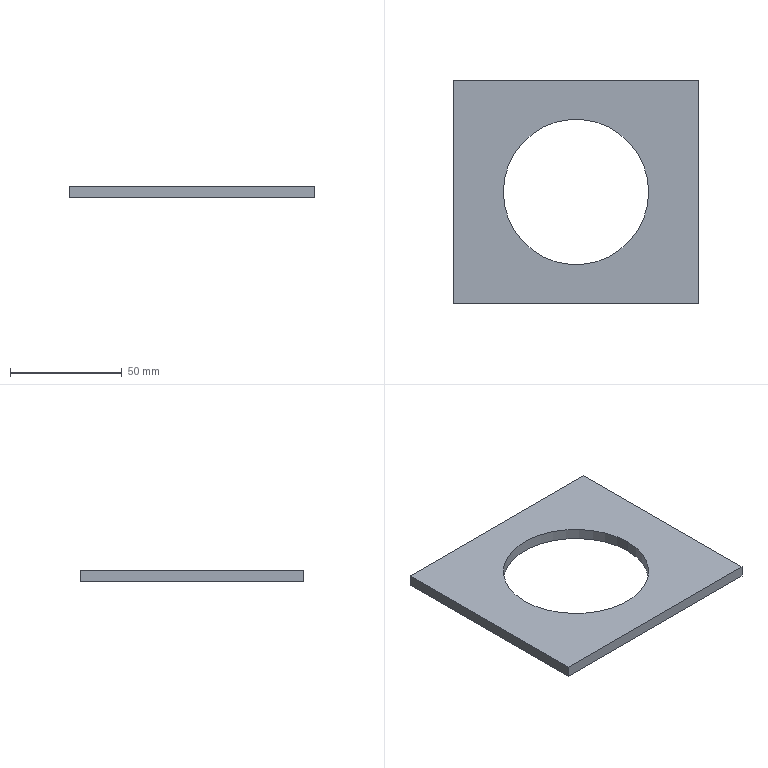Part | SolidWorks | features ICE 5, Extrusion 1 | 1 solid | 8 faces | box 110 x 100 x 5 mm | volume 38408 mm3 | plane 6 | cylinder 2 | commonest cylinder face diameters 65 x2
STEP:
#1=CARTESIAN_POINT('',(22.5,50.,0.));
#2=VERTEX_POINT('',#1);
#3=CARTESIAN_POINT('',(87.5,50.,0.));
#4=VERTEX_POINT('',#3);
#5=CARTESIAN_POINT('',(55.,50.,0.));
#6=DIRECTION('',(0.,0.,1.));
#7=DIRECTION('',(1.,0.,0.));
#8=AXIS2_PLACEMENT_3D('',#5,#6,#7);
#9=CIRCLE('',#8,32.5);
#10=EDGE_CURVE('',#2,#4,#9,.T.);
#11=ORIENTED_EDGE('',*,*,#10,.F.);
#12=CARTESIAN_POINT('',(22.5,50.,5.));
#13=VERTEX_POINT('',#12);
#14=CARTESIAN_POINT('',(22.5,50.,0.));
#15=DIRECTION('',(0.,0.,1.));
#16=VECTOR('',#15,1000.);
#17=LINE('',#14,#16);
#18=EDGE_CURVE('',#2,#13,#17,.T.);
#19=ORIENTED_EDGE('',*,*,#18,.T.);
#20=CARTESIAN_POINT('',(87.5,50.,5.));
#21=VERTEX_POINT('',#20);
#22=CARTESIAN_POINT('',(55.,50.,5.));
#23=DIRECTION('',(0.,0.,1.));
#24=DIRECTION('',(1.,0.,0.));
#25=AXIS2_PLACEMENT_3D('',#22,#23,#24);
#26=CIRCLE('',#25,32.5);
#27=EDGE_CURVE('',#13,#21,#26,.T.);
#28=ORIENTED_EDGE('',*,*,#27,.T.);
#29=CARTESIAN_POINT('',(87.5,50.,0.));
#30=DIRECTION('',(0.,0.,1.));
#31=VECTOR('',#30,1000.);
#32=LINE('',#29,#31);
#33=EDGE_CURVE('',#4,#21,#32,.T.);
#34=ORIENTED_EDGE('',*,*,#33,.F.);
#35=EDGE_LOOP('',(#11,#19,#28,#34));
#36=FACE_OUTER_BOUND('',#35,.T.);
#37=CARTESIAN_POINT('',(55.,50.,0.));
#38=DIRECTION('',(0.,0.,1.));
#39=DIRECTION('',(1.,0.,0.));
#40=AXIS2_PLACEMENT_3D('',#37,#38,#39);
#41=CYLINDRICAL_SURFACE('',#40,32.5);
#42=ADVANCED_FACE('',(#36),#41,.F.);
#43=CARTESIAN_POINT('',(0.,0.,0.));
#44=VERTEX_POINT('',#43);
#45=CARTESIAN_POINT('',(0.,0.,5.));
#46=VERTEX_POINT('',#45);
#47=CARTESIAN_POINT('',(0.,0.,0.));
#48=DIRECTION('',(0.,0.,1.));
#49=VECTOR('',#48,1000.);
#50=LINE('',#47,#49);
#51=EDGE_CURVE('',#44,#46,#50,.T.);
#52=ORIENTED_EDGE('',*,*,#51,.F.);
#53=CARTESIAN_POINT('',(110.,0.,0.));
#54=VERTEX_POINT('',#53);
#55=CARTESIAN_POINT('',(0.,0.,0.));
#56=DIRECTION('',(1.,0.,0.));
#57=VECTOR('',#56,1000.);
#58=LINE('',#55,#57);
#59=EDGE_CURVE('',#44,#54,#58,.T.);
#60=ORIENTED_EDGE('',*,*,#59,.T.);
#61=CARTESIAN_POINT('',(110.,0.,5.));
#62=VERTEX_POINT('',#61);
#63=CARTESIAN_POINT('',(110.,0.,5.));
#64=DIRECTION('',(0.,0.,-1.));
#65=VECTOR('',#64,1000.);
#66=LINE('',#63,#65);
#67=EDGE_CURVE('',#62,#54,#66,.T.);
#68=ORIENTED_EDGE('',*,*,#67,.F.);
#69=CARTESIAN_POINT('',(0.,0.,5.));
#70=DIRECTION('',(1.,0.,0.));
#71=VECTOR('',#70,1000.);
#72=LINE('',#69,#71);
#73=EDGE_CURVE('',#46,#62,#72,.T.);
#74=ORIENTED_EDGE('',*,*,#73,.F.);
#75=EDGE_LOOP('',(#52,#60,#68,#74));
#76=FACE_OUTER_BOUND('',#75,.T.);
#77=CARTESIAN_POINT('',(0.,0.,5.));
#78=DIRECTION('',(0.,1.,0.));
#79=DIRECTION('',(0.,0.,1.));
#80=AXIS2_PLACEMENT_3D('',#77,#78,#79);
#81=PLANE('',#80);
#82=ADVANCED_FACE('',(#76),#81,.F.);
#83=CARTESIAN_POINT('',(0.,100.,5.));
#84=VERTEX_POINT('',#83);
#85=CARTESIAN_POINT('',(0.,100.,0.));
#86=VERTEX_POINT('',#85);
#87=CARTESIAN_POINT('',(0.,100.,5.));
#88=DIRECTION('',(0.,0.,-1.));
#89=VECTOR('',#88,1000.);
#90=LINE('',#87,#89);
#91=EDGE_CURVE('',#84,#86,#90,.T.);
#92=ORIENTED_EDGE('',*,*,#91,.F.);
#93=CARTESIAN_POINT('',(110.,100.,5.));
#94=VERTEX_POINT('',#93);
#95=CARTESIAN_POINT('',(110.,100.,5.));
#96=DIRECTION('',(-1.,0.,0.));
#97=VECTOR('',#96,1000.);
#98=LINE('',#95,#97);
#99=EDGE_CURVE('',#94,#84,#98,.T.);
#100=ORIENTED_EDGE('',*,*,#99,.F.);
#101=CARTESIAN_POINT('',(110.,100.,0.));
#102=VERTEX_POINT('',#101);
#103=CARTESIAN_POINT('',(110.,100.,0.));
#104=DIRECTION('',(0.,0.,1.));
#105=VECTOR('',#104,1000.);
#106=LINE('',#103,#105);
#107=EDGE_CURVE('',#102,#94,#106,.T.);
#108=ORIENTED_EDGE('',*,*,#107,.F.);
#109=CARTESIAN_POINT('',(110.,100.,0.));
#110=DIRECTION('',(-1.,0.,0.));
#111=VECTOR('',#110,1000.);
#112=LINE('',#109,#111);
#113=EDGE_CURVE('',#102,#86,#112,.T.);
#114=ORIENTED_EDGE('',*,*,#113,.T.);
#115=EDGE_LOOP('',(#92,#100,#108,#114));
#116=FACE_OUTER_BOUND('',#115,.T.);
#117=CARTESIAN_POINT('',(110.,100.,5.));
#118=DIRECTION('',(0.,-1.,0.));
#119=DIRECTION('',(0.,0.,-1.));
#120=AXIS2_PLACEMENT_3D('',#117,#118,#119);
#121=PLANE('',#120);
#122=ADVANCED_FACE('',(#116),#121,.F.);
#123=CARTESIAN_POINT('',(55.,50.,5.));
#124=DIRECTION('',(0.,0.,1.));
#125=DIRECTION('',(1.,0.,0.));
#126=AXIS2_PLACEMENT_3D('',#123,#124,#125);
#127=CIRCLE('',#126,32.5);
#128=EDGE_CURVE('',#21,#13,#127,.T.);
#129=ORIENTED_EDGE('',*,*,#128,.F.);
#130=ORIENTED_EDGE('',*,*,#27,.F.);
#131=EDGE_LOOP('',(#129,#130));
#132=FACE_BOUND('',#131,.T.);
#133=ORIENTED_EDGE('',*,*,#99,.T.);
#134=CARTESIAN_POINT('',(0.,0.,5.));
#135=DIRECTION('',(0.,1.,0.));
#136=VECTOR('',#135,1000.);
#137=LINE('',#134,#136);
#138=EDGE_CURVE('',#46,#84,#137,.T.);
#139=ORIENTED_EDGE('',*,*,#138,.F.);
#140=ORIENTED_EDGE('',*,*,#73,.T.);
#141=CARTESIAN_POINT('',(110.,100.,5.));
#142=DIRECTION('',(0.,-1.,0.));
#143=VECTOR('',#142,1000.);
#144=LINE('',#141,#143);
#145=EDGE_CURVE('',#94,#62,#144,.T.);
#146=ORIENTED_EDGE('',*,*,#145,.F.);
#147=EDGE_LOOP('',(#133,#139,#140,#146));
#148=FACE_OUTER_BOUND('',#147,.T.);
#149=CARTESIAN_POINT('',(0.,0.,5.));
#150=DIRECTION('',(0.,0.,1.));
#151=DIRECTION('',(1.,0.,0.));
#152=AXIS2_PLACEMENT_3D('',#149,#150,#151);
#153=PLANE('',#152);
#154=ADVANCED_FACE('',(#132,#148),#153,.T.);
#155=CARTESIAN_POINT('',(55.,50.,0.));
#156=DIRECTION('',(0.,0.,1.));
#157=DIRECTION('',(1.,0.,0.));
#158=AXIS2_PLACEMENT_3D('',#155,#156,#157);
#159=CIRCLE('',#158,32.5);
#160=EDGE_CURVE('',#4,#2,#159,.T.);
#161=ORIENTED_EDGE('',*,*,#160,.T.);
#162=ORIENTED_EDGE('',*,*,#10,.T.);
#163=EDGE_LOOP('',(#161,#162));
#164=FACE_BOUND('',#163,.T.);
#165=CARTESIAN_POINT('',(0.,100.,0.));
#166=DIRECTION('',(0.,-1.,0.));
#167=VECTOR('',#166,1000.);
#168=LINE('',#165,#167);
#169=EDGE_CURVE('',#86,#44,#168,.T.);
#170=ORIENTED_EDGE('',*,*,#169,.F.);
#171=ORIENTED_EDGE('',*,*,#113,.F.);
#172=CARTESIAN_POINT('',(110.,0.,0.));
#173=DIRECTION('',(0.,1.,0.));
#174=VECTOR('',#173,1000.);
#175=LINE('',#172,#174);
#176=EDGE_CURVE('',#54,#102,#175,.T.);
#177=ORIENTED_EDGE('',*,*,#176,.F.);
#178=ORIENTED_EDGE('',*,*,#59,.F.);
#179=EDGE_LOOP('',(#170,#171,#177,#178));
#180=FACE_OUTER_BOUND('',#179,.T.);
#181=CARTESIAN_POINT('',(0.,0.,0.));
#182=DIRECTION('',(0.,0.,1.));
#183=DIRECTION('',(1.,0.,0.));
#184=AXIS2_PLACEMENT_3D('',#181,#182,#183);
#185=PLANE('',#184);
#186=ADVANCED_FACE('',(#164,#180),#185,.F.);
#187=ORIENTED_EDGE('',*,*,#18,.F.);
#188=ORIENTED_EDGE('',*,*,#160,.F.);
#189=ORIENTED_EDGE('',*,*,#33,.T.);
#190=ORIENTED_EDGE('',*,*,#128,.T.);
#191=EDGE_LOOP('',(#187,#188,#189,#190));
#192=FACE_OUTER_BOUND('',#191,.T.);
#193=CARTESIAN_POINT('',(55.,50.,0.));
#194=DIRECTION('',(0.,0.,1.));
#195=DIRECTION('',(1.,0.,0.));
#196=AXIS2_PLACEMENT_3D('',#193,#194,#195);
#197=CYLINDRICAL_SURFACE('',#196,32.5);
#198=ADVANCED_FACE('',(#192),#197,.F.);
#199=ORIENTED_EDGE('',*,*,#145,.T.);
#200=ORIENTED_EDGE('',*,*,#67,.T.);
#201=ORIENTED_EDGE('',*,*,#176,.T.);
#202=ORIENTED_EDGE('',*,*,#107,.T.);
#203=EDGE_LOOP('',(#199,#200,#201,#202));
#204=FACE_OUTER_BOUND('',#203,.T.);
#205=CARTESIAN_POINT('',(110.,0.,0.));
#206=DIRECTION('',(1.,0.,0.));
#207=DIRECTION('',(0.,0.,-1.));
#208=AXIS2_PLACEMENT_3D('',#205,#206,#207);
#209=PLANE('',#208);
#210=ADVANCED_FACE('',(#204),#209,.T.);
#211=ORIENTED_EDGE('',*,*,#138,.T.);
#212=ORIENTED_EDGE('',*,*,#91,.T.);
#213=ORIENTED_EDGE('',*,*,#169,.T.);
#214=ORIENTED_EDGE('',*,*,#51,.T.);
#215=EDGE_LOOP('',(#211,#212,#213,#214));
#216=FACE_OUTER_BOUND('',#215,.T.);
#217=CARTESIAN_POINT('',(0.,0.,0.));
#218=DIRECTION('',(-1.,0.,0.));
#219=DIRECTION('',(0.,0.,1.));
#220=AXIS2_PLACEMENT_3D('',#217,#218,#219);
#221=PLANE('',#220);
#222=ADVANCED_FACE('',(#216),#221,.T.);
#223=CLOSED_SHELL('',(#42,#82,#122,#154,#186,#198,#210,#222));
#224=MANIFOLD_SOLID_BREP('',#223);
#225=CARTESIAN_POINT('',(0.,0.,0.));
#226=DIRECTION('',(0.,0.,1.));
#227=DIRECTION('',(1.,0.,0.));
#228=AXIS2_PLACEMENT_3D('',#225,#226,#227);
#229=(LENGTH_UNIT()NAMED_UNIT(*)SI_UNIT(.MILLI.,.METRE.));
#230=UNCERTAINTY_MEASURE_WITH_UNIT(LENGTH_MEASURE(0.00001),#229,'','');
#231=(NAMED_UNIT(*)PLANE_ANGLE_UNIT()SI_UNIT($,.RADIAN.));
#232=(NAMED_UNIT(*)SI_UNIT($,.STERADIAN.)SOLID_ANGLE_UNIT());
#233=(GEOMETRIC_REPRESENTATION_CONTEXT(3)GLOBAL_UNCERTAINTY_ASSIGNED_CONTEXT((#230))GLOBAL_UNIT_ASSIGNED_CONTEXT((#229,#231,#232))REPRESENTATION_CONTEXT('',''));
#234=ADVANCED_BREP_SHAPE_REPRESENTATION('',(#224,#228),#233);